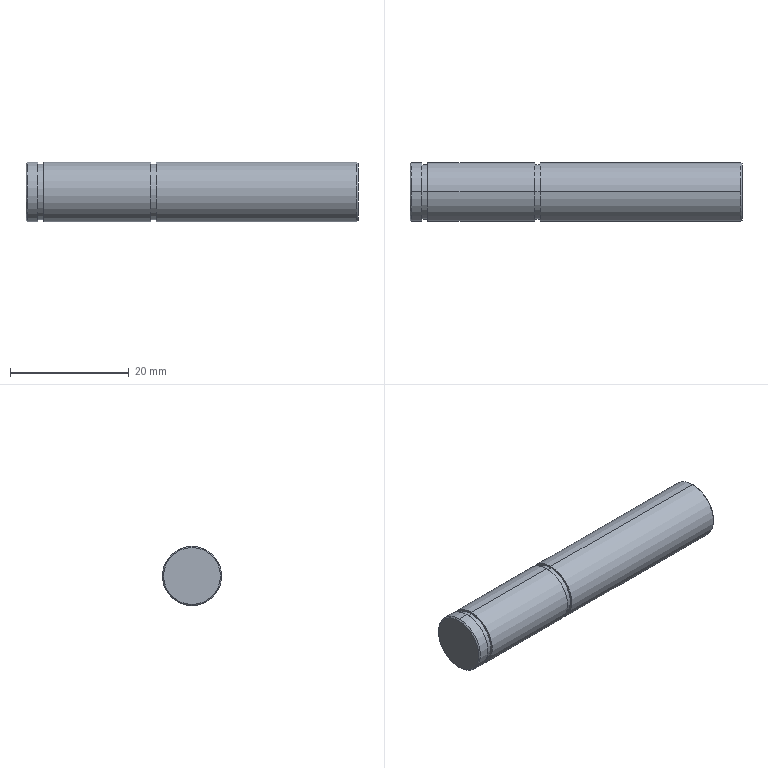Part | STEP file | Truc con lan | 1 solid | 20 faces | box 56 x 10 x 10 mm | volume 4376 mm3 | cylinder 10 | plane 6 | cone 4 | commonest cylinder face diameters 10 x6 9.3 x4
STEP:
#1=CARTESIAN_POINT('',(-56.,0.,4.8));
#2=VERTEX_POINT('',#1);
#3=CARTESIAN_POINT('',(-56.,0.,-4.8));
#4=VERTEX_POINT('',#3);
#5=CARTESIAN_POINT('',(-56.,0.,0.));
#6=DIRECTION('',(-1.,0.,0.));
#7=DIRECTION('',(0.,0.,-1.));
#8=AXIS2_PLACEMENT_3D('',#5,#6,#7);
#9=CIRCLE('',#8,4.8);
#10=EDGE_CURVE('',#2,#4,#9,.T.);
#11=ORIENTED_EDGE('',*,*,#10,.F.);
#12=CARTESIAN_POINT('',(-55.8,0.,5.));
#13=VERTEX_POINT('',#12);
#14=CARTESIAN_POINT('',(-56.,0.,4.8));
#15=DIRECTION('',(0.7071,0.,0.7071));
#16=VECTOR('',#15,1000.);
#17=LINE('',#14,#16);
#18=EDGE_CURVE('',#2,#13,#17,.T.);
#19=ORIENTED_EDGE('',*,*,#18,.T.);
#20=CARTESIAN_POINT('',(-55.8,0.,-5.));
#21=VERTEX_POINT('',#20);
#22=CARTESIAN_POINT('',(-55.8,0.,0.));
#23=DIRECTION('',(1.,0.,0.));
#24=DIRECTION('',(0.,0.,-1.));
#25=AXIS2_PLACEMENT_3D('',#22,#23,#24);
#26=CIRCLE('',#25,5.);
#27=EDGE_CURVE('',#21,#13,#26,.T.);
#28=ORIENTED_EDGE('',*,*,#27,.F.);
#29=CARTESIAN_POINT('',(-56.,0.,-4.8));
#30=DIRECTION('',(0.7071,0.,-0.7071));
#31=VECTOR('',#30,1000.);
#32=LINE('',#29,#31);
#33=EDGE_CURVE('',#4,#21,#32,.T.);
#34=ORIENTED_EDGE('',*,*,#33,.F.);
#35=EDGE_LOOP('',(#11,#19,#28,#34));
#36=FACE_OUTER_BOUND('',#35,.T.);
#37=CARTESIAN_POINT('',(-56.,0.,0.));
#38=DIRECTION('',(1.,0.,0.));
#39=DIRECTION('',(0.,0.,-1.));
#40=AXIS2_PLACEMENT_3D('',#37,#38,#39);
#41=CONICAL_SURFACE('',#40,4.8,0.7854);
#42=ADVANCED_FACE('',(#36),#41,.T.);
#43=CARTESIAN_POINT('',(0.,0.,-4.8));
#44=VERTEX_POINT('',#43);
#45=CARTESIAN_POINT('',(0.,0.,4.8));
#46=VERTEX_POINT('',#45);
#47=CARTESIAN_POINT('',(0.,0.,0.));
#48=DIRECTION('',(1.,0.,0.));
#49=DIRECTION('',(0.,0.,1.));
#50=AXIS2_PLACEMENT_3D('',#47,#48,#49);
#51=CIRCLE('',#50,4.8);
#52=EDGE_CURVE('',#44,#46,#51,.T.);
#53=ORIENTED_EDGE('',*,*,#52,.F.);
#54=CARTESIAN_POINT('',(-0.2,0.,-5.));
#55=VERTEX_POINT('',#54);
#56=CARTESIAN_POINT('',(-0.2,0.,-5.));
#57=DIRECTION('',(-0.7071,0.,-0.7071));
#58=VECTOR('',#57,1000.);
#59=LINE('',#56,#58);
#60=EDGE_CURVE('',#44,#55,#59,.T.);
#61=ORIENTED_EDGE('',*,*,#60,.T.);
#62=CARTESIAN_POINT('',(-0.2,0.,5.));
#63=VERTEX_POINT('',#62);
#64=CARTESIAN_POINT('',(-0.2,0.,0.));
#65=DIRECTION('',(-1.,0.,0.));
#66=DIRECTION('',(0.,0.,1.));
#67=AXIS2_PLACEMENT_3D('',#64,#65,#66);
#68=CIRCLE('',#67,5.);
#69=EDGE_CURVE('',#63,#55,#68,.T.);
#70=ORIENTED_EDGE('',*,*,#69,.F.);
#71=CARTESIAN_POINT('',(-0.2,0.,5.));
#72=DIRECTION('',(-0.7071,0.,0.7071));
#73=VECTOR('',#72,1000.);
#74=LINE('',#71,#73);
#75=EDGE_CURVE('',#46,#63,#74,.T.);
#76=ORIENTED_EDGE('',*,*,#75,.F.);
#77=EDGE_LOOP('',(#53,#61,#70,#76));
#78=FACE_OUTER_BOUND('',#77,.T.);
#79=CARTESIAN_POINT('',(-0.2,0.,0.));
#80=DIRECTION('',(-1.,0.,0.));
#81=DIRECTION('',(0.,0.,1.));
#82=AXIS2_PLACEMENT_3D('',#79,#80,#81);
#83=CONICAL_SURFACE('',#82,5.,0.7854);
#84=ADVANCED_FACE('',(#78),#83,.T.);
#85=CARTESIAN_POINT('',(-54.,0.,5.));
#86=VERTEX_POINT('',#85);
#87=CARTESIAN_POINT('',(-54.,0.,-5.));
#88=VERTEX_POINT('',#87);
#89=CARTESIAN_POINT('',(-54.,0.,0.));
#90=DIRECTION('',(-1.,0.,0.));
#91=DIRECTION('',(0.,0.,1.));
#92=AXIS2_PLACEMENT_3D('',#89,#90,#91);
#93=CIRCLE('',#92,5.);
#94=EDGE_CURVE('',#86,#88,#93,.T.);
#95=ORIENTED_EDGE('',*,*,#94,.T.);
#96=CARTESIAN_POINT('',(0.,0.,-5.));
#97=DIRECTION('',(-1.,0.,0.));
#98=VECTOR('',#97,1000.);
#99=LINE('',#96,#98);
#100=EDGE_CURVE('',#88,#21,#99,.T.);
#101=ORIENTED_EDGE('',*,*,#100,.T.);
#102=ORIENTED_EDGE('',*,*,#27,.T.);
#103=CARTESIAN_POINT('',(0.,0.,5.));
#104=DIRECTION('',(-1.,0.,0.));
#105=VECTOR('',#104,1000.);
#106=LINE('',#103,#105);
#107=EDGE_CURVE('',#86,#13,#106,.T.);
#108=ORIENTED_EDGE('',*,*,#107,.F.);
#109=EDGE_LOOP('',(#95,#101,#102,#108));
#110=FACE_OUTER_BOUND('',#109,.T.);
#111=CARTESIAN_POINT('',(0.,0.,0.));
#112=DIRECTION('',(-1.,0.,0.));
#113=DIRECTION('',(0.,0.,1.));
#114=AXIS2_PLACEMENT_3D('',#111,#112,#113);
#115=CYLINDRICAL_SURFACE('',#114,5.);
#116=ADVANCED_FACE('',(#110),#115,.T.);
#117=CARTESIAN_POINT('',(-53.,0.,4.65));
#118=VERTEX_POINT('',#117);
#119=CARTESIAN_POINT('',(-53.,0.,-4.65));
#120=VERTEX_POINT('',#119);
#121=CARTESIAN_POINT('',(-53.,0.,0.));
#122=DIRECTION('',(-1.,0.,0.));
#123=DIRECTION('',(0.,0.,1.));
#124=AXIS2_PLACEMENT_3D('',#121,#122,#123);
#125=CIRCLE('',#124,4.65);
#126=EDGE_CURVE('',#118,#120,#125,.T.);
#127=ORIENTED_EDGE('',*,*,#126,.T.);
#128=CARTESIAN_POINT('',(-54.,0.,-4.65));
#129=VERTEX_POINT('',#128);
#130=CARTESIAN_POINT('',(0.,0.,-4.65));
#131=DIRECTION('',(-1.,0.,0.));
#132=VECTOR('',#131,1000.);
#133=LINE('',#130,#132);
#134=EDGE_CURVE('',#120,#129,#133,.T.);
#135=ORIENTED_EDGE('',*,*,#134,.T.);
#136=CARTESIAN_POINT('',(-54.,0.,4.65));
#137=VERTEX_POINT('',#136);
#138=CARTESIAN_POINT('',(-54.,0.,0.));
#139=DIRECTION('',(-1.,0.,0.));
#140=DIRECTION('',(0.,0.,1.));
#141=AXIS2_PLACEMENT_3D('',#138,#139,#140);
#142=CIRCLE('',#141,4.65);
#143=EDGE_CURVE('',#137,#129,#142,.T.);
#144=ORIENTED_EDGE('',*,*,#143,.F.);
#145=CARTESIAN_POINT('',(0.,0.,4.65));
#146=DIRECTION('',(-1.,0.,0.));
#147=VECTOR('',#146,1000.);
#148=LINE('',#145,#147);
#149=EDGE_CURVE('',#118,#137,#148,.T.);
#150=ORIENTED_EDGE('',*,*,#149,.F.);
#151=EDGE_LOOP('',(#127,#135,#144,#150));
#152=FACE_OUTER_BOUND('',#151,.T.);
#153=CARTESIAN_POINT('',(0.,0.,0.));
#154=DIRECTION('',(-1.,0.,0.));
#155=DIRECTION('',(0.,0.,1.));
#156=AXIS2_PLACEMENT_3D('',#153,#154,#155);
#157=CYLINDRICAL_SURFACE('',#156,4.65);
#158=ADVANCED_FACE('',(#152),#157,.T.);
#159=CARTESIAN_POINT('',(-35.,0.,5.));
#160=VERTEX_POINT('',#159);
#161=CARTESIAN_POINT('',(-35.,0.,-5.));
#162=VERTEX_POINT('',#161);
#163=CARTESIAN_POINT('',(-35.,0.,0.));
#164=DIRECTION('',(-1.,0.,0.));
#165=DIRECTION('',(0.,0.,1.));
#166=AXIS2_PLACEMENT_3D('',#163,#164,#165);
#167=CIRCLE('',#166,5.);
#168=EDGE_CURVE('',#160,#162,#167,.T.);
#169=ORIENTED_EDGE('',*,*,#168,.T.);
#170=CARTESIAN_POINT('',(-53.,0.,-5.));
#171=VERTEX_POINT('',#170);
#172=CARTESIAN_POINT('',(0.,0.,-5.));
#173=DIRECTION('',(-1.,0.,0.));
#174=VECTOR('',#173,1000.);
#175=LINE('',#172,#174);
#176=EDGE_CURVE('',#162,#171,#175,.T.);
#177=ORIENTED_EDGE('',*,*,#176,.T.);
#178=CARTESIAN_POINT('',(-53.,0.,5.));
#179=VERTEX_POINT('',#178);
#180=CARTESIAN_POINT('',(-53.,0.,0.));
#181=DIRECTION('',(-1.,0.,0.));
#182=DIRECTION('',(0.,0.,1.));
#183=AXIS2_PLACEMENT_3D('',#180,#181,#182);
#184=CIRCLE('',#183,5.);
#185=EDGE_CURVE('',#179,#171,#184,.T.);
#186=ORIENTED_EDGE('',*,*,#185,.F.);
#187=CARTESIAN_POINT('',(0.,0.,5.));
#188=DIRECTION('',(-1.,0.,0.));
#189=VECTOR('',#188,1000.);
#190=LINE('',#187,#189);
#191=EDGE_CURVE('',#160,#179,#190,.T.);
#192=ORIENTED_EDGE('',*,*,#191,.F.);
#193=EDGE_LOOP('',(#169,#177,#186,#192));
#194=FACE_OUTER_BOUND('',#193,.T.);
#195=CARTESIAN_POINT('',(0.,0.,0.));
#196=DIRECTION('',(-1.,0.,0.));
#197=DIRECTION('',(0.,0.,1.));
#198=AXIS2_PLACEMENT_3D('',#195,#196,#197);
#199=CYLINDRICAL_SURFACE('',#198,5.);
#200=ADVANCED_FACE('',(#194),#199,.T.);
#201=CARTESIAN_POINT('',(-34.,0.,4.65));
#202=VERTEX_POINT('',#201);
#203=CARTESIAN_POINT('',(-34.,0.,-4.65));
#204=VERTEX_POINT('',#203);
#205=CARTESIAN_POINT('',(-34.,0.,0.));
#206=DIRECTION('',(-1.,0.,0.));
#207=DIRECTION('',(0.,0.,1.));
#208=AXIS2_PLACEMENT_3D('',#205,#206,#207);
#209=CIRCLE('',#208,4.65);
#210=EDGE_CURVE('',#202,#204,#209,.T.);
#211=ORIENTED_EDGE('',*,*,#210,.T.);
#212=CARTESIAN_POINT('',(-35.,0.,-4.65));
#213=VERTEX_POINT('',#212);
#214=CARTESIAN_POINT('',(0.,0.,-4.65));
#215=DIRECTION('',(-1.,0.,0.));
#216=VECTOR('',#215,1000.);
#217=LINE('',#214,#216);
#218=EDGE_CURVE('',#204,#213,#217,.T.);
#219=ORIENTED_EDGE('',*,*,#218,.T.);
#220=CARTESIAN_POINT('',(-35.,0.,4.65));
#221=VERTEX_POINT('',#220);
#222=CARTESIAN_POINT('',(-35.,0.,0.));
#223=DIRECTION('',(-1.,0.,0.));
#224=DIRECTION('',(0.,0.,1.));
#225=AXIS2_PLACEMENT_3D('',#222,#223,#224);
#226=CIRCLE('',#225,4.65);
#227=EDGE_CURVE('',#221,#213,#226,.T.);
#228=ORIENTED_EDGE('',*,*,#227,.F.);
#229=CARTESIAN_POINT('',(0.,0.,4.65));
#230=DIRECTION('',(-1.,0.,0.));
#231=VECTOR('',#230,1000.);
#232=LINE('',#229,#231);
#233=EDGE_CURVE('',#202,#221,#232,.T.);
#234=ORIENTED_EDGE('',*,*,#233,.F.);
#235=EDGE_LOOP('',(#211,#219,#228,#234));
#236=FACE_OUTER_BOUND('',#235,.T.);
#237=CARTESIAN_POINT('',(0.,0.,0.));
#238=DIRECTION('',(-1.,0.,0.));
#239=DIRECTION('',(0.,0.,1.));
#240=AXIS2_PLACEMENT_3D('',#237,#238,#239);
#241=CYLINDRICAL_SURFACE('',#240,4.65);
#242=ADVANCED_FACE('',(#236),#241,.T.);
#243=ORIENTED_EDGE('',*,*,#69,.T.);
#244=CARTESIAN_POINT('',(-34.,0.,-5.));
#245=VERTEX_POINT('',#244);
#246=CARTESIAN_POINT('',(0.,0.,-5.));
#247=DIRECTION('',(-1.,0.,0.));
#248=VECTOR('',#247,1000.);
#249=LINE('',#246,#248);
#250=EDGE_CURVE('',#55,#245,#249,.T.);
#251=ORIENTED_EDGE('',*,*,#250,.T.);
#252=CARTESIAN_POINT('',(-34.,0.,5.));
#253=VERTEX_POINT('',#252);
#254=CARTESIAN_POINT('',(-34.,0.,0.));
#255=DIRECTION('',(-1.,0.,0.));
#256=DIRECTION('',(0.,0.,1.));
#257=AXIS2_PLACEMENT_3D('',#254,#255,#256);
#258=CIRCLE('',#257,5.);
#259=EDGE_CURVE('',#253,#245,#258,.T.);
#260=ORIENTED_EDGE('',*,*,#259,.F.);
#261=CARTESIAN_POINT('',(0.,0.,5.));
#262=DIRECTION('',(-1.,0.,0.));
#263=VECTOR('',#262,1000.);
#264=LINE('',#261,#263);
#265=EDGE_CURVE('',#63,#253,#264,.T.);
#266=ORIENTED_EDGE('',*,*,#265,.F.);
#267=EDGE_LOOP('',(#243,#251,#260,#266));
#268=FACE_OUTER_BOUND('',#267,.T.);
#269=CARTESIAN_POINT('',(0.,0.,0.));
#270=DIRECTION('',(-1.,0.,0.));
#271=DIRECTION('',(0.,0.,1.));
#272=AXIS2_PLACEMENT_3D('',#269,#270,#271);
#273=CYLINDRICAL_SURFACE('',#272,5.);
#274=ADVANCED_FACE('',(#268),#273,.T.);
#275=CARTESIAN_POINT('',(0.,0.,0.));
#276=DIRECTION('',(1.,0.,0.));
#277=DIRECTION('',(0.,0.,1.));
#278=AXIS2_PLACEMENT_3D('',#275,#276,#277);
#279=CIRCLE('',#278,4.8);
#280=EDGE_CURVE('',#46,#44,#279,.T.);
#281=ORIENTED_EDGE('',*,*,#280,.T.);
#282=ORIENTED_EDGE('',*,*,#52,.T.);
#283=EDGE_LOOP('',(#281,#282));
#284=FACE_OUTER_BOUND('',#283,.T.);
#285=CARTESIAN_POINT('',(0.,0.,0.));
#286=DIRECTION('',(-1.,0.,0.));
#287=DIRECTION('',(0.,0.,1.));
#288=AXIS2_PLACEMENT_3D('',#285,#286,#287);
#289=PLANE('',#288);
#290=ADVANCED_FACE('',(#284),#289,.F.);
#291=ORIENTED_EDGE('',*,*,#250,.F.);
#292=CARTESIAN_POINT('',(-0.2,0.,0.));
#293=DIRECTION('',(-1.,0.,0.));
#294=DIRECTION('',(0.,0.,1.));
#295=AXIS2_PLACEMENT_3D('',#292,#293,#294);
#296=CIRCLE('',#295,5.);
#297=EDGE_CURVE('',#55,#63,#296,.T.);
#298=ORIENTED_EDGE('',*,*,#297,.T.);
#299=ORIENTED_EDGE('',*,*,#265,.T.);
#300=CARTESIAN_POINT('',(-34.,0.,0.));
#301=DIRECTION('',(-1.,0.,0.));
#302=DIRECTION('',(0.,0.,1.));
#303=AXIS2_PLACEMENT_3D('',#300,#301,#302);
#304=CIRCLE('',#303,5.);
#305=EDGE_CURVE('',#245,#253,#304,.T.);
#306=ORIENTED_EDGE('',*,*,#305,.F.);
#307=EDGE_LOOP('',(#291,#298,#299,#306));
#308=FACE_OUTER_BOUND('',#307,.T.);
#309=CARTESIAN_POINT('',(0.,0.,0.));
#310=DIRECTION('',(-1.,0.,0.));
#311=DIRECTION('',(0.,0.,1.));
#312=AXIS2_PLACEMENT_3D('',#309,#310,#311);
#313=CYLINDRICAL_SURFACE('',#312,5.);
#314=ADVANCED_FACE('',(#308),#313,.T.);
#315=ORIENTED_EDGE('',*,*,#210,.F.);
#316=CARTESIAN_POINT('',(-34.,0.,0.));
#317=DIRECTION('',(-1.,0.,0.));
#318=DIRECTION('',(0.,0.,1.));
#319=AXIS2_PLACEMENT_3D('',#316,#317,#318);
#320=CIRCLE('',#319,4.65);
#321=EDGE_CURVE('',#204,#202,#320,.T.);
#322=ORIENTED_EDGE('',*,*,#321,.F.);
#323=EDGE_LOOP('',(#315,#322));
#324=FACE_BOUND('',#323,.T.);
#325=ORIENTED_EDGE('',*,*,#259,.T.);
#326=ORIENTED_EDGE('',*,*,#305,.T.);
#327=EDGE_LOOP('',(#325,#326));
#328=FACE_OUTER_BOUND('',#327,.T.);
#329=CARTESIAN_POINT('',(-34.,4.65,0.));
#330=DIRECTION('',(1.,0.,0.));
#331=DIRECTION('',(0.,0.,-1.));
#332=AXIS2_PLACEMENT_3D('',#329,#330,#331);
#333=PLANE('',#332);
#334=ADVANCED_FACE('',(#324,#328),#333,.F.);
#335=ORIENTED_EDGE('',*,*,#218,.F.);
#336=ORIENTED_EDGE('',*,*,#321,.T.);
#337=ORIENTED_EDGE('',*,*,#233,.T.);
#338=CARTESIAN_POINT('',(-35.,0.,0.));
#339=DIRECTION('',(-1.,0.,0.));
#340=DIRECTION('',(0.,0.,1.));
#341=AXIS2_PLACEMENT_3D('',#338,#339,#340);
#342=CIRCLE('',#341,4.65);
#343=EDGE_CURVE('',#213,#221,#342,.T.);
#344=ORIENTED_EDGE('',*,*,#343,.F.);
#345=EDGE_LOOP('',(#335,#336,#337,#344));
#346=FACE_OUTER_BOUND('',#345,.T.);
#347=CARTESIAN_POINT('',(0.,0.,0.));
#348=DIRECTION('',(-1.,0.,0.));
#349=DIRECTION('',(0.,0.,1.));
#350=AXIS2_PLACEMENT_3D('',#347,#348,#349);
#351=CYLINDRICAL_SURFACE('',#350,4.65);
#352=ADVANCED_FACE('',(#346),#351,.T.);
#353=ORIENTED_EDGE('',*,*,#168,.F.);
#354=CARTESIAN_POINT('',(-35.,0.,0.));
#355=DIRECTION('',(-1.,0.,0.));
#356=DIRECTION('',(0.,0.,1.));
#357=AXIS2_PLACEMENT_3D('',#354,#355,#356);
#358=CIRCLE('',#357,5.);
#359=EDGE_CURVE('',#162,#160,#358,.T.);
#360=ORIENTED_EDGE('',*,*,#359,.F.);
#361=EDGE_LOOP('',(#353,#360));
#362=FACE_OUTER_BOUND('',#361,.T.);
#363=ORIENTED_EDGE('',*,*,#227,.T.);
#364=ORIENTED_EDGE('',*,*,#343,.T.);
#365=EDGE_LOOP('',(#363,#364));
#366=FACE_BOUND('',#365,.T.);
#367=CARTESIAN_POINT('',(-35.,5.,0.));
#368=DIRECTION('',(-1.,0.,0.));
#369=DIRECTION('',(0.,0.,1.));
#370=AXIS2_PLACEMENT_3D('',#367,#368,#369);
#371=PLANE('',#370);
#372=ADVANCED_FACE('',(#362,#366),#371,.F.);
#373=ORIENTED_EDGE('',*,*,#176,.F.);
#374=ORIENTED_EDGE('',*,*,#359,.T.);
#375=ORIENTED_EDGE('',*,*,#191,.T.);
#376=CARTESIAN_POINT('',(-53.,0.,0.));
#377=DIRECTION('',(-1.,0.,0.));
#378=DIRECTION('',(0.,0.,1.));
#379=AXIS2_PLACEMENT_3D('',#376,#377,#378);
#380=CIRCLE('',#379,5.);
#381=EDGE_CURVE('',#171,#179,#380,.T.);
#382=ORIENTED_EDGE('',*,*,#381,.F.);
#383=EDGE_LOOP('',(#373,#374,#375,#382));
#384=FACE_OUTER_BOUND('',#383,.T.);
#385=CARTESIAN_POINT('',(0.,0.,0.));
#386=DIRECTION('',(-1.,0.,0.));
#387=DIRECTION('',(0.,0.,1.));
#388=AXIS2_PLACEMENT_3D('',#385,#386,#387);
#389=CYLINDRICAL_SURFACE('',#388,5.);
#390=ADVANCED_FACE('',(#384),#389,.T.);
#391=ORIENTED_EDGE('',*,*,#126,.F.);
#392=CARTESIAN_POINT('',(-53.,0.,0.));
#393=DIRECTION('',(-1.,0.,0.));
#394=DIRECTION('',(0.,0.,1.));
#395=AXIS2_PLACEMENT_3D('',#392,#393,#394);
#396=CIRCLE('',#395,4.65);
#397=EDGE_CURVE('',#120,#118,#396,.T.);
#398=ORIENTED_EDGE('',*,*,#397,.F.);
#399=EDGE_LOOP('',(#391,#398));
#400=FACE_BOUND('',#399,.T.);
#401=ORIENTED_EDGE('',*,*,#185,.T.);
#402=ORIENTED_EDGE('',*,*,#381,.T.);
#403=EDGE_LOOP('',(#401,#402));
#404=FACE_OUTER_BOUND('',#403,.T.);
#405=CARTESIAN_POINT('',(-53.,5.,0.));
#406=DIRECTION('',(1.,0.,0.));
#407=DIRECTION('',(0.,0.,-1.));
#408=AXIS2_PLACEMENT_3D('',#405,#406,#407);
#409=PLANE('',#408);
#410=ADVANCED_FACE('',(#400,#404),#409,.F.);
#411=ORIENTED_EDGE('',*,*,#134,.F.);
#412=ORIENTED_EDGE('',*,*,#397,.T.);
#413=ORIENTED_EDGE('',*,*,#149,.T.);
#414=CARTESIAN_POINT('',(-54.,0.,0.));
#415=DIRECTION('',(-1.,0.,0.));
#416=DIRECTION('',(0.,0.,1.));
#417=AXIS2_PLACEMENT_3D('',#414,#415,#416);
#418=CIRCLE('',#417,4.65);
#419=EDGE_CURVE('',#129,#137,#418,.T.);
#420=ORIENTED_EDGE('',*,*,#419,.F.);
#421=EDGE_LOOP('',(#411,#412,#413,#420));
#422=FACE_OUTER_BOUND('',#421,.T.);
#423=CARTESIAN_POINT('',(0.,0.,0.));
#424=DIRECTION('',(-1.,0.,0.));
#425=DIRECTION('',(0.,0.,1.));
#426=AXIS2_PLACEMENT_3D('',#423,#424,#425);
#427=CYLINDRICAL_SURFACE('',#426,4.65);
#428=ADVANCED_FACE('',(#422),#427,.T.);
#429=ORIENTED_EDGE('',*,*,#94,.F.);
#430=CARTESIAN_POINT('',(-54.,0.,0.));
#431=DIRECTION('',(-1.,0.,0.));
#432=DIRECTION('',(0.,0.,1.));
#433=AXIS2_PLACEMENT_3D('',#430,#431,#432);
#434=CIRCLE('',#433,5.);
#435=EDGE_CURVE('',#88,#86,#434,.T.);
#436=ORIENTED_EDGE('',*,*,#435,.F.);
#437=EDGE_LOOP('',(#429,#436));
#438=FACE_OUTER_BOUND('',#437,.T.);
#439=ORIENTED_EDGE('',*,*,#143,.T.);
#440=ORIENTED_EDGE('',*,*,#419,.T.);
#441=EDGE_LOOP('',(#439,#440));
#442=FACE_BOUND('',#441,.T.);
#443=CARTESIAN_POINT('',(-54.,4.65,0.));
#444=DIRECTION('',(-1.,0.,0.));
#445=DIRECTION('',(0.,0.,1.));
#446=AXIS2_PLACEMENT_3D('',#443,#444,#445);
#447=PLANE('',#446);
#448=ADVANCED_FACE('',(#438,#442),#447,.F.);
#449=ORIENTED_EDGE('',*,*,#100,.F.);
#450=ORIENTED_EDGE('',*,*,#435,.T.);
#451=ORIENTED_EDGE('',*,*,#107,.T.);
#452=CARTESIAN_POINT('',(-55.8,0.,0.));
#453=DIRECTION('',(1.,0.,0.));
#454=DIRECTION('',(0.,0.,-1.));
#455=AXIS2_PLACEMENT_3D('',#452,#453,#454);
#456=CIRCLE('',#455,5.);
#457=EDGE_CURVE('',#13,#21,#456,.T.);
#458=ORIENTED_EDGE('',*,*,#457,.T.);
#459=EDGE_LOOP('',(#449,#450,#451,#458));
#460=FACE_OUTER_BOUND('',#459,.T.);
#461=CARTESIAN_POINT('',(0.,0.,0.));
#462=DIRECTION('',(-1.,0.,0.));
#463=DIRECTION('',(0.,0.,1.));
#464=AXIS2_PLACEMENT_3D('',#461,#462,#463);
#465=CYLINDRICAL_SURFACE('',#464,5.);
#466=ADVANCED_FACE('',(#460),#465,.T.);
#467=CARTESIAN_POINT('',(-56.,0.,0.));
#468=DIRECTION('',(-1.,0.,0.));
#469=DIRECTION('',(0.,0.,-1.));
#470=AXIS2_PLACEMENT_3D('',#467,#468,#469);
#471=CIRCLE('',#470,4.8);
#472=EDGE_CURVE('',#4,#2,#471,.T.);
#473=ORIENTED_EDGE('',*,*,#472,.T.);
#474=ORIENTED_EDGE('',*,*,#10,.T.);
#475=EDGE_LOOP('',(#473,#474));
#476=FACE_OUTER_BOUND('',#475,.T.);
#477=CARTESIAN_POINT('',(-56.,5.,0.));
#478=DIRECTION('',(1.,0.,0.));
#479=DIRECTION('',(0.,0.,-1.));
#480=AXIS2_PLACEMENT_3D('',#477,#478,#479);
#481=PLANE('',#480);
#482=ADVANCED_FACE('',(#476),#481,.F.);
#483=ORIENTED_EDGE('',*,*,#60,.F.);
#484=ORIENTED_EDGE('',*,*,#280,.F.);
#485=ORIENTED_EDGE('',*,*,#75,.T.);
#486=ORIENTED_EDGE('',*,*,#297,.F.);
#487=EDGE_LOOP('',(#483,#484,#485,#486));
#488=FACE_OUTER_BOUND('',#487,.T.);
#489=CARTESIAN_POINT('',(-0.2,0.,0.));
#490=DIRECTION('',(-1.,0.,0.));
#491=DIRECTION('',(0.,0.,1.));
#492=AXIS2_PLACEMENT_3D('',#489,#490,#491);
#493=CONICAL_SURFACE('',#492,5.,0.7854);
#494=ADVANCED_FACE('',(#488),#493,.T.);
#495=ORIENTED_EDGE('',*,*,#18,.F.);
#496=ORIENTED_EDGE('',*,*,#472,.F.);
#497=ORIENTED_EDGE('',*,*,#33,.T.);
#498=ORIENTED_EDGE('',*,*,#457,.F.);
#499=EDGE_LOOP('',(#495,#496,#497,#498));
#500=FACE_OUTER_BOUND('',#499,.T.);
#501=CARTESIAN_POINT('',(-56.,0.,0.));
#502=DIRECTION('',(1.,0.,0.));
#503=DIRECTION('',(0.,0.,-1.));
#504=AXIS2_PLACEMENT_3D('',#501,#502,#503);
#505=CONICAL_SURFACE('',#504,4.8,0.7854);
#506=ADVANCED_FACE('',(#500),#505,.T.);
#507=CLOSED_SHELL('',(#42,#84,#116,#158,#200,#242,#274,#290,#314,#334,#352,#372,#390,#410,#428,#448,#466,#482,#494,#506));
#508=MANIFOLD_SOLID_BREP('',#507);
#509=CARTESIAN_POINT('',(0.,0.,0.));
#510=DIRECTION('',(0.,0.,1.));
#511=DIRECTION('',(1.,0.,0.));
#512=AXIS2_PLACEMENT_3D('',#509,#510,#511);
#513=(LENGTH_UNIT()NAMED_UNIT(*)SI_UNIT(.MILLI.,.METRE.));
#514=UNCERTAINTY_MEASURE_WITH_UNIT(LENGTH_MEASURE(0.00001),#513,'','');
#515=(NAMED_UNIT(*)PLANE_ANGLE_UNIT()SI_UNIT($,.RADIAN.));
#516=(NAMED_UNIT(*)SI_UNIT($,.STERADIAN.)SOLID_ANGLE_UNIT());
#517=(GEOMETRIC_REPRESENTATION_CONTEXT(3)GLOBAL_UNCERTAINTY_ASSIGNED_CONTEXT((#514))GLOBAL_UNIT_ASSIGNED_CONTEXT((#513,#515,#516))REPRESENTATION_CONTEXT('',''));
#518=ADVANCED_BREP_SHAPE_REPRESENTATION('',(#508,#512),#517);